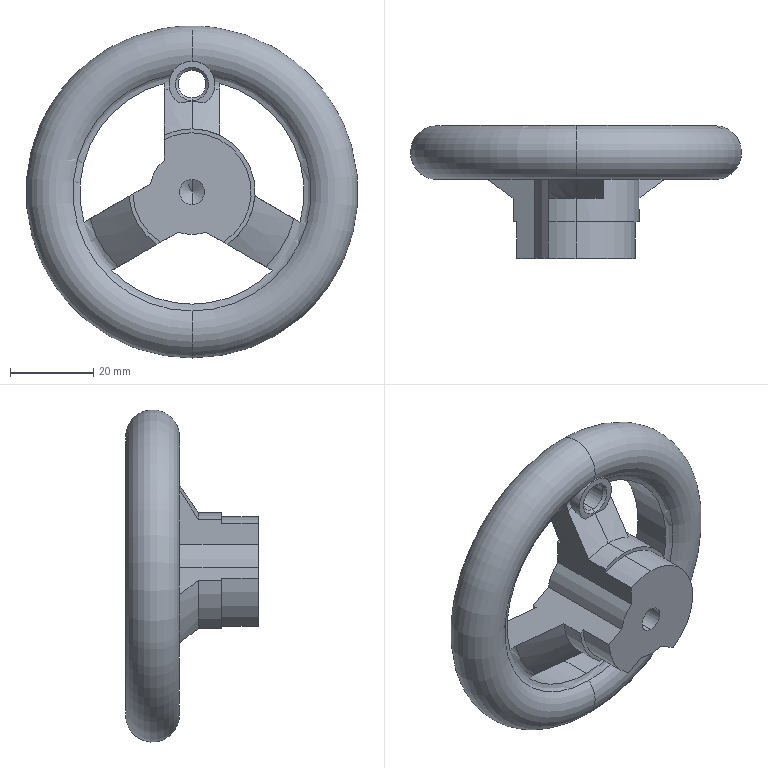Part | SolidWorks | features RefAxis 9, 3DProfileFeature 3, Revolution 3, RevCut 2, CirPattern 1, ICE 1 | 1 solid | 52 faces | box 80 x 32 x 80 mm | volume 48291 mm3 | cylinder 22 | cone 14 | plane 12 | torus 4 | commonest cylinder face diameters 30.4 x5 54 x4 11 x3 20.4 x3 28.5 x3 6 x2